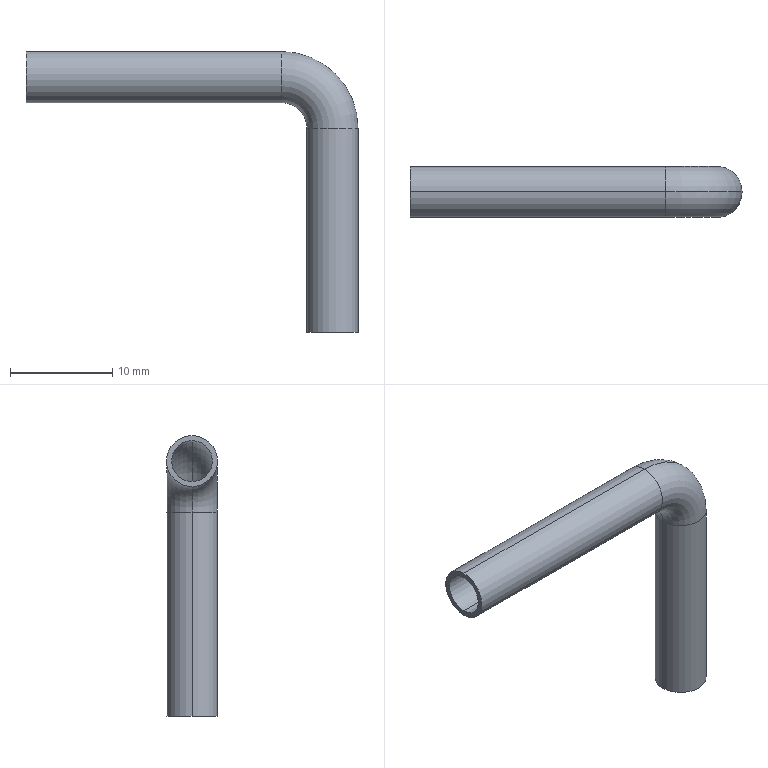Part | SolidWorks | features Sweep 1 | 1 solid | 14 faces | box 32.5 x 5 x 27.5 mm | volume 373.603 mm3 | cylinder 8 | torus 4 | plane 2 | commonest cylinder face diameters 4 x4 5 x4
STEP:
#1=CARTESIAN_POINT('',(2.,0.,20.));
#2=VERTEX_POINT('',#1);
#3=CARTESIAN_POINT('',(-2.,0.,20.));
#4=VERTEX_POINT('',#3);
#5=CARTESIAN_POINT('',(0.,0.,20.));
#6=DIRECTION('',(0.,0.,1.));
#7=DIRECTION('',(1.,0.,0.));
#8=AXIS2_PLACEMENT_3D('',#5,#6,#7);
#9=CIRCLE('',#8,2.);
#10=EDGE_CURVE('',#2,#4,#9,.T.);
#11=ORIENTED_EDGE('',*,*,#10,.F.);
#12=CARTESIAN_POINT('',(-5.,0.,27.));
#13=VERTEX_POINT('',#12);
#14=CARTESIAN_POINT('',(-5.,0.,20.));
#15=DIRECTION('',(0.,-1.,0.));
#16=DIRECTION('',(0.,0.,-1.));
#17=AXIS2_PLACEMENT_3D('',#14,#15,#16);
#18=CIRCLE('',#17,7.);
#19=EDGE_CURVE('',#2,#13,#18,.T.);
#20=ORIENTED_EDGE('',*,*,#19,.T.);
#21=CARTESIAN_POINT('',(-5.,0.,23.));
#22=VERTEX_POINT('',#21);
#23=CARTESIAN_POINT('',(-5.,0.,25.));
#24=DIRECTION('',(-1.,0.,0.));
#25=DIRECTION('',(0.,0.,1.));
#26=AXIS2_PLACEMENT_3D('',#23,#24,#25);
#27=CIRCLE('',#26,2.);
#28=EDGE_CURVE('',#13,#22,#27,.T.);
#29=ORIENTED_EDGE('',*,*,#28,.T.);
#30=CARTESIAN_POINT('',(-5.,0.,20.));
#31=DIRECTION('',(0.,-1.,0.));
#32=DIRECTION('',(0.,0.,-1.));
#33=AXIS2_PLACEMENT_3D('',#30,#31,#32);
#34=CIRCLE('',#33,3.);
#35=EDGE_CURVE('',#4,#22,#34,.T.);
#36=ORIENTED_EDGE('',*,*,#35,.F.);
#37=EDGE_LOOP('',(#11,#20,#29,#36));
#38=FACE_OUTER_BOUND('',#37,.T.);
#39=CARTESIAN_POINT('',(-5.,0.,20.));
#40=DIRECTION('',(0.,-1.,0.));
#41=DIRECTION('',(0.,0.,-1.));
#42=AXIS2_PLACEMENT_3D('',#39,#40,#41);
#43=TOROIDAL_SURFACE('',#42,5.,2.);
#44=ADVANCED_FACE('',(#38),#43,.F.);
#45=CARTESIAN_POINT('',(-2.5,0.,20.));
#46=VERTEX_POINT('',#45);
#47=CARTESIAN_POINT('',(2.5,0.,20.));
#48=VERTEX_POINT('',#47);
#49=CARTESIAN_POINT('',(0.,0.,20.));
#50=DIRECTION('',(0.,0.,1.));
#51=DIRECTION('',(1.,0.,0.));
#52=AXIS2_PLACEMENT_3D('',#49,#50,#51);
#53=CIRCLE('',#52,2.5);
#54=EDGE_CURVE('',#46,#48,#53,.T.);
#55=ORIENTED_EDGE('',*,*,#54,.T.);
#56=CARTESIAN_POINT('',(-5.,0.,27.5));
#57=VERTEX_POINT('',#56);
#58=CARTESIAN_POINT('',(-5.,0.,20.));
#59=DIRECTION('',(0.,-1.,0.));
#60=DIRECTION('',(0.,0.,-1.));
#61=AXIS2_PLACEMENT_3D('',#58,#59,#60);
#62=CIRCLE('',#61,7.5);
#63=EDGE_CURVE('',#48,#57,#62,.T.);
#64=ORIENTED_EDGE('',*,*,#63,.T.);
#65=CARTESIAN_POINT('',(-5.,0.,22.5));
#66=VERTEX_POINT('',#65);
#67=CARTESIAN_POINT('',(-5.,0.,25.));
#68=DIRECTION('',(-1.,0.,0.));
#69=DIRECTION('',(0.,0.,1.));
#70=AXIS2_PLACEMENT_3D('',#67,#68,#69);
#71=CIRCLE('',#70,2.5);
#72=EDGE_CURVE('',#66,#57,#71,.T.);
#73=ORIENTED_EDGE('',*,*,#72,.F.);
#74=CARTESIAN_POINT('',(-5.,0.,20.));
#75=DIRECTION('',(0.,-1.,0.));
#76=DIRECTION('',(0.,0.,-1.));
#77=AXIS2_PLACEMENT_3D('',#74,#75,#76);
#78=CIRCLE('',#77,2.5);
#79=EDGE_CURVE('',#46,#66,#78,.T.);
#80=ORIENTED_EDGE('',*,*,#79,.F.);
#81=EDGE_LOOP('',(#55,#64,#73,#80));
#82=FACE_OUTER_BOUND('',#81,.T.);
#83=CARTESIAN_POINT('',(-5.,0.,20.));
#84=DIRECTION('',(0.,-1.,0.));
#85=DIRECTION('',(0.,0.,-1.));
#86=AXIS2_PLACEMENT_3D('',#83,#84,#85);
#87=TOROIDAL_SURFACE('',#86,5.,2.5);
#88=ADVANCED_FACE('',(#82),#87,.T.);
#89=CARTESIAN_POINT('',(0.,0.,20.));
#90=DIRECTION('',(0.,0.,1.));
#91=DIRECTION('',(1.,0.,0.));
#92=AXIS2_PLACEMENT_3D('',#89,#90,#91);
#93=CIRCLE('',#92,2.5);
#94=EDGE_CURVE('',#48,#46,#93,.T.);
#95=ORIENTED_EDGE('',*,*,#94,.F.);
#96=CARTESIAN_POINT('',(2.5,0.,0.));
#97=VERTEX_POINT('',#96);
#98=CARTESIAN_POINT('',(2.5,0.,20.));
#99=DIRECTION('',(0.,0.,-1.));
#100=VECTOR('',#99,1000.);
#101=LINE('',#98,#100);
#102=EDGE_CURVE('',#48,#97,#101,.T.);
#103=ORIENTED_EDGE('',*,*,#102,.T.);
#104=CARTESIAN_POINT('',(-2.5,0.,0.));
#105=VERTEX_POINT('',#104);
#106=CARTESIAN_POINT('',(0.,0.,0.));
#107=DIRECTION('',(0.,0.,1.));
#108=DIRECTION('',(1.,0.,0.));
#109=AXIS2_PLACEMENT_3D('',#106,#107,#108);
#110=CIRCLE('',#109,2.5);
#111=EDGE_CURVE('',#97,#105,#110,.T.);
#112=ORIENTED_EDGE('',*,*,#111,.T.);
#113=CARTESIAN_POINT('',(-2.5,0.,20.));
#114=DIRECTION('',(0.,0.,-1.));
#115=VECTOR('',#114,1000.);
#116=LINE('',#113,#115);
#117=EDGE_CURVE('',#46,#105,#116,.T.);
#118=ORIENTED_EDGE('',*,*,#117,.F.);
#119=EDGE_LOOP('',(#95,#103,#112,#118));
#120=FACE_OUTER_BOUND('',#119,.T.);
#121=CARTESIAN_POINT('',(0.,0.,20.));
#122=DIRECTION('',(0.,0.,-1.));
#123=DIRECTION('',(-1.,0.,0.));
#124=AXIS2_PLACEMENT_3D('',#121,#122,#123);
#125=CYLINDRICAL_SURFACE('',#124,2.5);
#126=ADVANCED_FACE('',(#120),#125,.T.);
#127=CARTESIAN_POINT('',(0.,0.,20.));
#128=DIRECTION('',(0.,0.,1.));
#129=DIRECTION('',(1.,0.,0.));
#130=AXIS2_PLACEMENT_3D('',#127,#128,#129);
#131=CIRCLE('',#130,2.);
#132=EDGE_CURVE('',#4,#2,#131,.T.);
#133=ORIENTED_EDGE('',*,*,#132,.T.);
#134=CARTESIAN_POINT('',(2.,0.,0.));
#135=VERTEX_POINT('',#134);
#136=CARTESIAN_POINT('',(2.,0.,20.));
#137=DIRECTION('',(0.,0.,-1.));
#138=VECTOR('',#137,1000.);
#139=LINE('',#136,#138);
#140=EDGE_CURVE('',#2,#135,#139,.T.);
#141=ORIENTED_EDGE('',*,*,#140,.T.);
#142=CARTESIAN_POINT('',(-2.,0.,0.));
#143=VERTEX_POINT('',#142);
#144=CARTESIAN_POINT('',(0.,0.,0.));
#145=DIRECTION('',(0.,0.,1.));
#146=DIRECTION('',(1.,0.,0.));
#147=AXIS2_PLACEMENT_3D('',#144,#145,#146);
#148=CIRCLE('',#147,2.);
#149=EDGE_CURVE('',#143,#135,#148,.T.);
#150=ORIENTED_EDGE('',*,*,#149,.F.);
#151=CARTESIAN_POINT('',(-2.,0.,20.));
#152=DIRECTION('',(0.,0.,-1.));
#153=VECTOR('',#152,1000.);
#154=LINE('',#151,#153);
#155=EDGE_CURVE('',#4,#143,#154,.T.);
#156=ORIENTED_EDGE('',*,*,#155,.F.);
#157=EDGE_LOOP('',(#133,#141,#150,#156));
#158=FACE_OUTER_BOUND('',#157,.T.);
#159=CARTESIAN_POINT('',(0.,0.,20.));
#160=DIRECTION('',(0.,0.,-1.));
#161=DIRECTION('',(-1.,0.,0.));
#162=AXIS2_PLACEMENT_3D('',#159,#160,#161);
#163=CYLINDRICAL_SURFACE('',#162,2.);
#164=ADVANCED_FACE('',(#158),#163,.F.);
#165=CARTESIAN_POINT('',(-5.,0.,25.));
#166=DIRECTION('',(-1.,0.,0.));
#167=DIRECTION('',(0.,0.,1.));
#168=AXIS2_PLACEMENT_3D('',#165,#166,#167);
#169=CIRCLE('',#168,2.);
#170=EDGE_CURVE('',#22,#13,#169,.T.);
#171=ORIENTED_EDGE('',*,*,#170,.F.);
#172=CARTESIAN_POINT('',(-30.,0.,23.));
#173=VERTEX_POINT('',#172);
#174=CARTESIAN_POINT('',(-5.,0.,23.));
#175=DIRECTION('',(-1.,0.,0.));
#176=VECTOR('',#175,1000.);
#177=LINE('',#174,#176);
#178=EDGE_CURVE('',#22,#173,#177,.T.);
#179=ORIENTED_EDGE('',*,*,#178,.T.);
#180=CARTESIAN_POINT('',(-30.,0.,27.));
#181=VERTEX_POINT('',#180);
#182=CARTESIAN_POINT('',(-30.,0.,25.));
#183=DIRECTION('',(-1.,0.,0.));
#184=DIRECTION('',(0.,0.,1.));
#185=AXIS2_PLACEMENT_3D('',#182,#183,#184);
#186=CIRCLE('',#185,2.);
#187=EDGE_CURVE('',#173,#181,#186,.T.);
#188=ORIENTED_EDGE('',*,*,#187,.T.);
#189=CARTESIAN_POINT('',(-5.,0.,27.));
#190=DIRECTION('',(-1.,0.,0.));
#191=VECTOR('',#190,1000.);
#192=LINE('',#189,#191);
#193=EDGE_CURVE('',#13,#181,#192,.T.);
#194=ORIENTED_EDGE('',*,*,#193,.F.);
#195=EDGE_LOOP('',(#171,#179,#188,#194));
#196=FACE_OUTER_BOUND('',#195,.T.);
#197=CARTESIAN_POINT('',(-5.,0.,25.));
#198=DIRECTION('',(-1.,0.,0.));
#199=DIRECTION('',(0.,0.,1.));
#200=AXIS2_PLACEMENT_3D('',#197,#198,#199);
#201=CYLINDRICAL_SURFACE('',#200,2.);
#202=ADVANCED_FACE('',(#196),#201,.F.);
#203=CARTESIAN_POINT('',(-5.,0.,25.));
#204=DIRECTION('',(-1.,0.,0.));
#205=DIRECTION('',(0.,0.,1.));
#206=AXIS2_PLACEMENT_3D('',#203,#204,#205);
#207=CIRCLE('',#206,2.5);
#208=EDGE_CURVE('',#57,#66,#207,.T.);
#209=ORIENTED_EDGE('',*,*,#208,.T.);
#210=CARTESIAN_POINT('',(-30.,0.,22.5));
#211=VERTEX_POINT('',#210);
#212=CARTESIAN_POINT('',(-5.,0.,22.5));
#213=DIRECTION('',(-1.,0.,0.));
#214=VECTOR('',#213,1000.);
#215=LINE('',#212,#214);
#216=EDGE_CURVE('',#66,#211,#215,.T.);
#217=ORIENTED_EDGE('',*,*,#216,.T.);
#218=CARTESIAN_POINT('',(-30.,0.,27.5));
#219=VERTEX_POINT('',#218);
#220=CARTESIAN_POINT('',(-30.,0.,25.));
#221=DIRECTION('',(-1.,0.,0.));
#222=DIRECTION('',(0.,0.,1.));
#223=AXIS2_PLACEMENT_3D('',#220,#221,#222);
#224=CIRCLE('',#223,2.5);
#225=EDGE_CURVE('',#219,#211,#224,.T.);
#226=ORIENTED_EDGE('',*,*,#225,.F.);
#227=CARTESIAN_POINT('',(-5.,0.,27.5));
#228=DIRECTION('',(-1.,0.,0.));
#229=VECTOR('',#228,1000.);
#230=LINE('',#227,#229);
#231=EDGE_CURVE('',#57,#219,#230,.T.);
#232=ORIENTED_EDGE('',*,*,#231,.F.);
#233=EDGE_LOOP('',(#209,#217,#226,#232));
#234=FACE_OUTER_BOUND('',#233,.T.);
#235=CARTESIAN_POINT('',(-5.,0.,25.));
#236=DIRECTION('',(-1.,0.,0.));
#237=DIRECTION('',(0.,0.,1.));
#238=AXIS2_PLACEMENT_3D('',#235,#236,#237);
#239=CYLINDRICAL_SURFACE('',#238,2.5);
#240=ADVANCED_FACE('',(#234),#239,.T.);
#241=ORIENTED_EDGE('',*,*,#216,.F.);
#242=ORIENTED_EDGE('',*,*,#72,.T.);
#243=ORIENTED_EDGE('',*,*,#231,.T.);
#244=CARTESIAN_POINT('',(-30.,0.,25.));
#245=DIRECTION('',(-1.,0.,0.));
#246=DIRECTION('',(0.,0.,1.));
#247=AXIS2_PLACEMENT_3D('',#244,#245,#246);
#248=CIRCLE('',#247,2.5);
#249=EDGE_CURVE('',#211,#219,#248,.T.);
#250=ORIENTED_EDGE('',*,*,#249,.F.);
#251=EDGE_LOOP('',(#241,#242,#243,#250));
#252=FACE_OUTER_BOUND('',#251,.T.);
#253=CARTESIAN_POINT('',(-5.,0.,25.));
#254=DIRECTION('',(-1.,0.,0.));
#255=DIRECTION('',(0.,0.,1.));
#256=AXIS2_PLACEMENT_3D('',#253,#254,#255);
#257=CYLINDRICAL_SURFACE('',#256,2.5);
#258=ADVANCED_FACE('',(#252),#257,.T.);
#259=ORIENTED_EDGE('',*,*,#178,.F.);
#260=ORIENTED_EDGE('',*,*,#28,.F.);
#261=ORIENTED_EDGE('',*,*,#193,.T.);
#262=CARTESIAN_POINT('',(-30.,0.,25.));
#263=DIRECTION('',(-1.,0.,0.));
#264=DIRECTION('',(0.,0.,1.));
#265=AXIS2_PLACEMENT_3D('',#262,#263,#264);
#266=CIRCLE('',#265,2.);
#267=EDGE_CURVE('',#181,#173,#266,.T.);
#268=ORIENTED_EDGE('',*,*,#267,.T.);
#269=EDGE_LOOP('',(#259,#260,#261,#268));
#270=FACE_OUTER_BOUND('',#269,.T.);
#271=CARTESIAN_POINT('',(-5.,0.,25.));
#272=DIRECTION('',(-1.,0.,0.));
#273=DIRECTION('',(0.,0.,1.));
#274=AXIS2_PLACEMENT_3D('',#271,#272,#273);
#275=CYLINDRICAL_SURFACE('',#274,2.);
#276=ADVANCED_FACE('',(#270),#275,.F.);
#277=ORIENTED_EDGE('',*,*,#63,.F.);
#278=ORIENTED_EDGE('',*,*,#94,.T.);
#279=ORIENTED_EDGE('',*,*,#79,.T.);
#280=ORIENTED_EDGE('',*,*,#208,.F.);
#281=EDGE_LOOP('',(#277,#278,#279,#280));
#282=FACE_OUTER_BOUND('',#281,.T.);
#283=CARTESIAN_POINT('',(-5.,0.,20.));
#284=DIRECTION('',(0.,-1.,0.));
#285=DIRECTION('',(0.,0.,-1.));
#286=AXIS2_PLACEMENT_3D('',#283,#284,#285);
#287=TOROIDAL_SURFACE('',#286,5.,2.5);
#288=ADVANCED_FACE('',(#282),#287,.T.);
#289=ORIENTED_EDGE('',*,*,#19,.F.);
#290=ORIENTED_EDGE('',*,*,#132,.F.);
#291=ORIENTED_EDGE('',*,*,#35,.T.);
#292=ORIENTED_EDGE('',*,*,#170,.T.);
#293=EDGE_LOOP('',(#289,#290,#291,#292));
#294=FACE_OUTER_BOUND('',#293,.T.);
#295=CARTESIAN_POINT('',(-5.,0.,20.));
#296=DIRECTION('',(0.,-1.,0.));
#297=DIRECTION('',(0.,0.,-1.));
#298=AXIS2_PLACEMENT_3D('',#295,#296,#297);
#299=TOROIDAL_SURFACE('',#298,5.,2.);
#300=ADVANCED_FACE('',(#294),#299,.F.);
#301=ORIENTED_EDGE('',*,*,#140,.F.);
#302=ORIENTED_EDGE('',*,*,#10,.T.);
#303=ORIENTED_EDGE('',*,*,#155,.T.);
#304=CARTESIAN_POINT('',(0.,0.,0.));
#305=DIRECTION('',(0.,0.,1.));
#306=DIRECTION('',(1.,0.,0.));
#307=AXIS2_PLACEMENT_3D('',#304,#305,#306);
#308=CIRCLE('',#307,2.);
#309=EDGE_CURVE('',#135,#143,#308,.T.);
#310=ORIENTED_EDGE('',*,*,#309,.F.);
#311=EDGE_LOOP('',(#301,#302,#303,#310));
#312=FACE_OUTER_BOUND('',#311,.T.);
#313=CARTESIAN_POINT('',(0.,0.,20.));
#314=DIRECTION('',(0.,0.,-1.));
#315=DIRECTION('',(-1.,0.,0.));
#316=AXIS2_PLACEMENT_3D('',#313,#314,#315);
#317=CYLINDRICAL_SURFACE('',#316,2.);
#318=ADVANCED_FACE('',(#312),#317,.F.);
#319=ORIENTED_EDGE('',*,*,#102,.F.);
#320=ORIENTED_EDGE('',*,*,#54,.F.);
#321=ORIENTED_EDGE('',*,*,#117,.T.);
#322=CARTESIAN_POINT('',(0.,0.,0.));
#323=DIRECTION('',(0.,0.,1.));
#324=DIRECTION('',(1.,0.,0.));
#325=AXIS2_PLACEMENT_3D('',#322,#323,#324);
#326=CIRCLE('',#325,2.5);
#327=EDGE_CURVE('',#105,#97,#326,.T.);
#328=ORIENTED_EDGE('',*,*,#327,.T.);
#329=EDGE_LOOP('',(#319,#320,#321,#328));
#330=FACE_OUTER_BOUND('',#329,.T.);
#331=CARTESIAN_POINT('',(0.,0.,20.));
#332=DIRECTION('',(0.,0.,-1.));
#333=DIRECTION('',(-1.,0.,0.));
#334=AXIS2_PLACEMENT_3D('',#331,#332,#333);
#335=CYLINDRICAL_SURFACE('',#334,2.5);
#336=ADVANCED_FACE('',(#330),#335,.T.);
#337=ORIENTED_EDGE('',*,*,#267,.F.);
#338=ORIENTED_EDGE('',*,*,#187,.F.);
#339=EDGE_LOOP('',(#337,#338));
#340=FACE_BOUND('',#339,.T.);
#341=ORIENTED_EDGE('',*,*,#225,.T.);
#342=ORIENTED_EDGE('',*,*,#249,.T.);
#343=EDGE_LOOP('',(#341,#342));
#344=FACE_OUTER_BOUND('',#343,.T.);
#345=CARTESIAN_POINT('',(-30.,0.,25.));
#346=DIRECTION('',(-1.,0.,0.));
#347=DIRECTION('',(0.,0.,1.));
#348=AXIS2_PLACEMENT_3D('',#345,#346,#347);
#349=PLANE('',#348);
#350=ADVANCED_FACE('',(#340,#344),#349,.T.);
#351=ORIENTED_EDGE('',*,*,#149,.T.);
#352=ORIENTED_EDGE('',*,*,#309,.T.);
#353=EDGE_LOOP('',(#351,#352));
#354=FACE_BOUND('',#353,.T.);
#355=ORIENTED_EDGE('',*,*,#327,.F.);
#356=ORIENTED_EDGE('',*,*,#111,.F.);
#357=EDGE_LOOP('',(#355,#356));
#358=FACE_OUTER_BOUND('',#357,.T.);
#359=CARTESIAN_POINT('',(0.,0.,0.));
#360=DIRECTION('',(0.,0.,1.));
#361=DIRECTION('',(1.,0.,0.));
#362=AXIS2_PLACEMENT_3D('',#359,#360,#361);
#363=PLANE('',#362);
#364=ADVANCED_FACE('',(#354,#358),#363,.F.);
#365=CLOSED_SHELL('',(#44,#88,#126,#164,#202,#240,#258,#276,#288,#300,#318,#336,#350,#364));
#366=MANIFOLD_SOLID_BREP('',#365);
#367=CARTESIAN_POINT('',(0.,0.,0.));
#368=DIRECTION('',(0.,0.,1.));
#369=DIRECTION('',(1.,0.,0.));
#370=AXIS2_PLACEMENT_3D('',#367,#368,#369);
#371=(LENGTH_UNIT()NAMED_UNIT(*)SI_UNIT(.MILLI.,.METRE.));
#372=UNCERTAINTY_MEASURE_WITH_UNIT(LENGTH_MEASURE(0.00001),#371,'','');
#373=(NAMED_UNIT(*)PLANE_ANGLE_UNIT()SI_UNIT($,.RADIAN.));
#374=(NAMED_UNIT(*)SI_UNIT($,.STERADIAN.)SOLID_ANGLE_UNIT());
#375=(GEOMETRIC_REPRESENTATION_CONTEXT(3)GLOBAL_UNCERTAINTY_ASSIGNED_CONTEXT((#372))GLOBAL_UNIT_ASSIGNED_CONTEXT((#371,#373,#374))REPRESENTATION_CONTEXT('',''));
#376=ADVANCED_BREP_SHAPE_REPRESENTATION('',(#366,#370),#375);